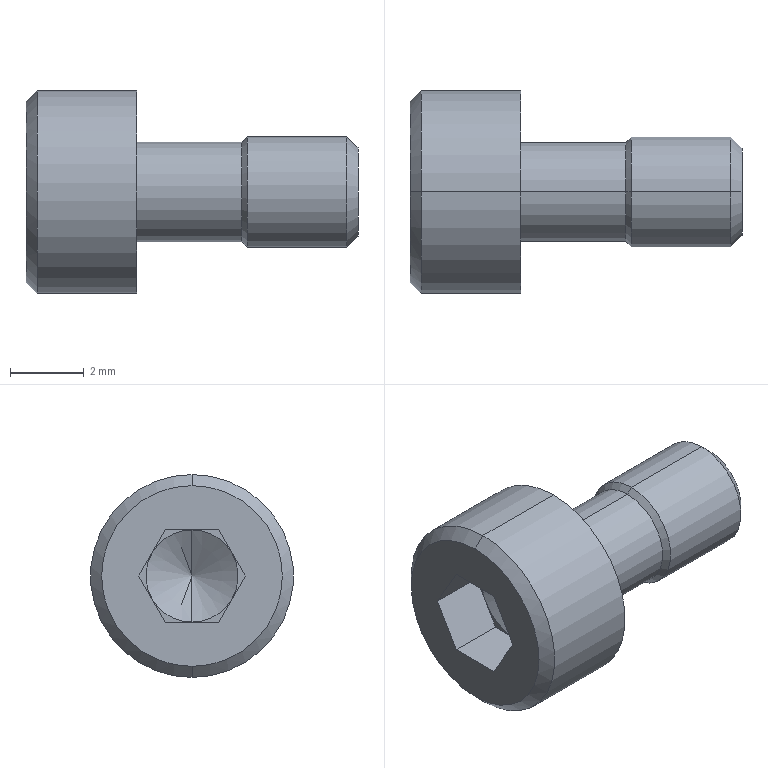Part | STEP file | 0244_Z_014_SCBS3-6_1 | 1 solid | 29 faces | box 9 x 5.5 x 5.5 mm | volume 99.208 mm3 | plane 15 | cone 8 | cylinder 6 | commonest cylinder face diameters 2.693 x2 3 x2 5.5 x2